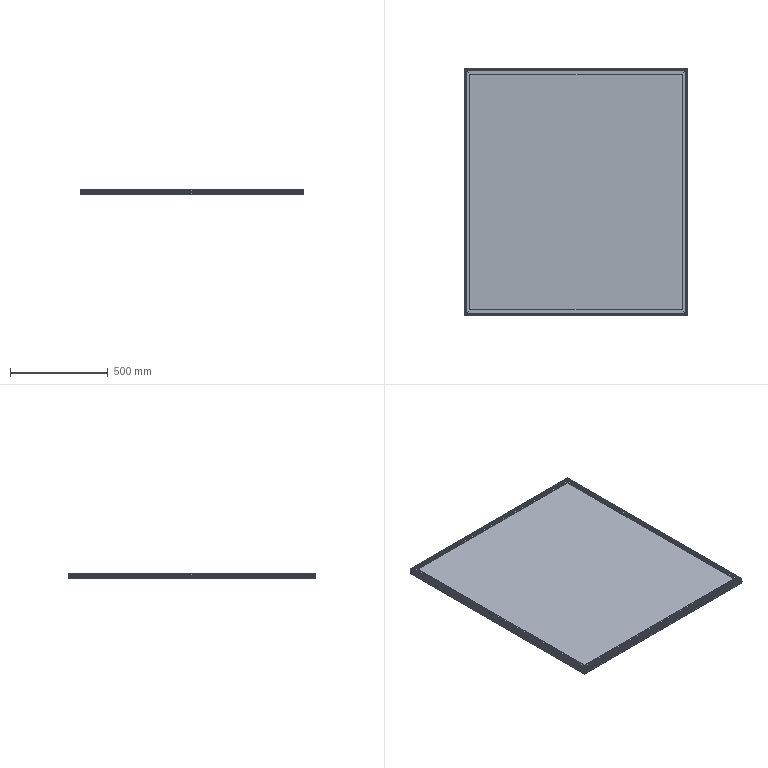Part | SolidWorks | features ICE 1, WeldMemberFeat 1, WeldmentFeature 1 | 5 solids | 272 faces | box 1140 x 1260 x 30 mm | volume 23522260 mm3 | plane 222 | cylinder 50 | commonest cylinder face diameters 0.4 x26 2 x16 1 x8